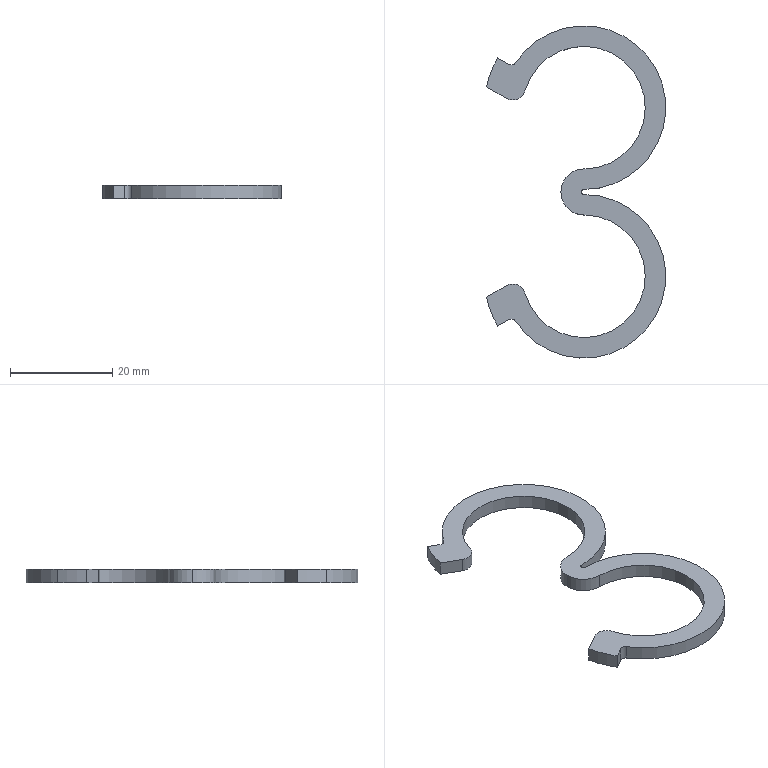Part | SolidWorks | features Extrusion 1 | 1 solid | 20 faces | box 35.068 x 65 x 2.7 mm | volume 1587 mm3 | cylinder 14 | plane 6 | commonest cylinder face diameters 1 x2 2 x2 5 x2 9 x2 24 x2 32 x2
STEP:
#1=CARTESIAN_POINT('',(-0.5,0.,2.7));
#2=VERTEX_POINT('',#1);
#3=CARTESIAN_POINT('',(0.,0.5,2.7));
#4=VERTEX_POINT('',#3);
#5=CARTESIAN_POINT('',(0.,0.,2.7));
#6=DIRECTION('',(0.,0.,-1.));
#7=DIRECTION('',(1.,0.,0.));
#8=AXIS2_PLACEMENT_3D('',#5,#6,#7);
#9=CIRCLE('',#8,0.5);
#10=EDGE_CURVE('',#2,#4,#9,.T.);
#11=ORIENTED_EDGE('',*,*,#10,.F.);
#12=CARTESIAN_POINT('',(-0.5,0.,0.));
#13=VERTEX_POINT('',#12);
#14=CARTESIAN_POINT('',(-0.5,0.,2.7));
#15=DIRECTION('',(0.,0.,-1.));
#16=VECTOR('',#15,1000.);
#17=LINE('',#14,#16);
#18=EDGE_CURVE('',#2,#13,#17,.T.);
#19=ORIENTED_EDGE('',*,*,#18,.T.);
#20=CARTESIAN_POINT('',(0.,0.5,0.));
#21=VERTEX_POINT('',#20);
#22=CARTESIAN_POINT('',(0.,0.,0.));
#23=DIRECTION('',(0.,0.,-1.));
#24=DIRECTION('',(1.,0.,0.));
#25=AXIS2_PLACEMENT_3D('',#22,#23,#24);
#26=CIRCLE('',#25,0.5);
#27=EDGE_CURVE('',#13,#21,#26,.T.);
#28=ORIENTED_EDGE('',*,*,#27,.T.);
#29=CARTESIAN_POINT('',(0.,0.5,2.7));
#30=DIRECTION('',(0.,0.,-1.));
#31=VECTOR('',#30,1000.);
#32=LINE('',#29,#31);
#33=EDGE_CURVE('',#4,#21,#32,.T.);
#34=ORIENTED_EDGE('',*,*,#33,.F.);
#35=EDGE_LOOP('',(#11,#19,#28,#34));
#36=FACE_OUTER_BOUND('',#35,.T.);
#37=CARTESIAN_POINT('',(0.,0.,2.7));
#38=DIRECTION('',(0.,0.,-1.));
#39=DIRECTION('',(-1.,0.,0.));
#40=AXIS2_PLACEMENT_3D('',#37,#38,#39);
#41=CYLINDRICAL_SURFACE('',#40,0.5);
#42=ADVANCED_FACE('',(#36),#41,.F.);
#43=CARTESIAN_POINT('',(-4.5,0.,2.7));
#44=VERTEX_POINT('',#43);
#45=CARTESIAN_POINT('',(0.,-4.5,2.7));
#46=VERTEX_POINT('',#45);
#47=CARTESIAN_POINT('',(0.,0.,2.7));
#48=DIRECTION('',(0.,0.,1.));
#49=DIRECTION('',(1.,0.,0.));
#50=AXIS2_PLACEMENT_3D('',#47,#48,#49);
#51=CIRCLE('',#50,4.5);
#52=EDGE_CURVE('',#44,#46,#51,.T.);
#53=ORIENTED_EDGE('',*,*,#52,.F.);
#54=CARTESIAN_POINT('',(-4.5,0.,0.));
#55=VERTEX_POINT('',#54);
#56=CARTESIAN_POINT('',(-4.5,0.,2.7));
#57=DIRECTION('',(0.,0.,-1.));
#58=VECTOR('',#57,1000.);
#59=LINE('',#56,#58);
#60=EDGE_CURVE('',#44,#55,#59,.T.);
#61=ORIENTED_EDGE('',*,*,#60,.T.);
#62=CARTESIAN_POINT('',(0.,-4.5,0.));
#63=VERTEX_POINT('',#62);
#64=CARTESIAN_POINT('',(0.,0.,0.));
#65=DIRECTION('',(0.,0.,1.));
#66=DIRECTION('',(1.,0.,0.));
#67=AXIS2_PLACEMENT_3D('',#64,#65,#66);
#68=CIRCLE('',#67,4.5);
#69=EDGE_CURVE('',#55,#63,#68,.T.);
#70=ORIENTED_EDGE('',*,*,#69,.T.);
#71=CARTESIAN_POINT('',(0.,-4.5,2.7));
#72=DIRECTION('',(0.,0.,-1.));
#73=VECTOR('',#72,1000.);
#74=LINE('',#71,#73);
#75=EDGE_CURVE('',#46,#63,#74,.T.);
#76=ORIENTED_EDGE('',*,*,#75,.F.);
#77=EDGE_LOOP('',(#53,#61,#70,#76));
#78=FACE_OUTER_BOUND('',#77,.T.);
#79=CARTESIAN_POINT('',(0.,0.,2.7));
#80=DIRECTION('',(0.,0.,-1.));
#81=DIRECTION('',(-1.,0.,0.));
#82=AXIS2_PLACEMENT_3D('',#79,#80,#81);
#83=CYLINDRICAL_SURFACE('',#82,4.5);
#84=ADVANCED_FACE('',(#78),#83,.T.);
#85=CARTESIAN_POINT('',(-16.887,26.25,0.));
#86=VERTEX_POINT('',#85);
#87=CARTESIAN_POINT('',(-19.068,20.581,0.));
#88=VERTEX_POINT('',#87);
#89=CARTESIAN_POINT('',(0.,16.5,0.));
#90=DIRECTION('',(0.,0.,1.));
#91=DIRECTION('',(1.,0.,0.));
#92=AXIS2_PLACEMENT_3D('',#89,#90,#91);
#93=CIRCLE('',#92,19.5);
#94=EDGE_CURVE('',#86,#88,#93,.T.);
#95=ORIENTED_EDGE('',*,*,#94,.T.);
#96=CARTESIAN_POINT('',(-19.068,20.581,2.7));
#97=VERTEX_POINT('',#96);
#98=CARTESIAN_POINT('',(-19.068,20.581,2.7));
#99=DIRECTION('',(0.,0.,-1.));
#100=VECTOR('',#99,1000.);
#101=LINE('',#98,#100);
#102=EDGE_CURVE('',#97,#88,#101,.T.);
#103=ORIENTED_EDGE('',*,*,#102,.F.);
#104=CARTESIAN_POINT('',(-16.887,26.25,2.7));
#105=VERTEX_POINT('',#104);
#106=CARTESIAN_POINT('',(0.,16.5,2.7));
#107=DIRECTION('',(0.,0.,1.));
#108=DIRECTION('',(1.,0.,0.));
#109=AXIS2_PLACEMENT_3D('',#106,#107,#108);
#110=CIRCLE('',#109,19.5);
#111=EDGE_CURVE('',#105,#97,#110,.T.);
#112=ORIENTED_EDGE('',*,*,#111,.F.);
#113=CARTESIAN_POINT('',(-16.887,26.25,2.7));
#114=DIRECTION('',(0.,0.,-1.));
#115=VECTOR('',#114,1000.);
#116=LINE('',#113,#115);
#117=EDGE_CURVE('',#105,#86,#116,.T.);
#118=ORIENTED_EDGE('',*,*,#117,.T.);
#119=EDGE_LOOP('',(#95,#103,#112,#118));
#120=FACE_OUTER_BOUND('',#119,.T.);
#121=CARTESIAN_POINT('',(0.,16.5,2.7));
#122=DIRECTION('',(0.,0.,-1.));
#123=DIRECTION('',(-1.,0.,0.));
#124=AXIS2_PLACEMENT_3D('',#121,#122,#123);
#125=CYLINDRICAL_SURFACE('',#124,19.5);
#126=ADVANCED_FACE('',(#120),#125,.T.);
#127=CARTESIAN_POINT('',(-15.186,18.339,0.));
#128=VERTEX_POINT('',#127);
#129=CARTESIAN_POINT('',(-15.186,18.339,0.));
#130=DIRECTION('',(0.866,-0.5,0.));
#131=VECTOR('',#130,1000.);
#132=LINE('',#129,#131);
#133=EDGE_CURVE('',#88,#128,#132,.T.);
#134=ORIENTED_EDGE('',*,*,#133,.T.);
#135=CARTESIAN_POINT('',(-15.186,18.339,2.7));
#136=VERTEX_POINT('',#135);
#137=CARTESIAN_POINT('',(-15.186,18.339,2.7));
#138=DIRECTION('',(0.,0.,-1.));
#139=VECTOR('',#138,1000.);
#140=LINE('',#137,#139);
#141=EDGE_CURVE('',#136,#128,#140,.T.);
#142=ORIENTED_EDGE('',*,*,#141,.F.);
#143=CARTESIAN_POINT('',(-15.186,18.339,2.7));
#144=DIRECTION('',(0.866,-0.5,0.));
#145=VECTOR('',#144,1000.);
#146=LINE('',#143,#145);
#147=EDGE_CURVE('',#97,#136,#146,.T.);
#148=ORIENTED_EDGE('',*,*,#147,.F.);
#149=ORIENTED_EDGE('',*,*,#102,.T.);
#150=EDGE_LOOP('',(#134,#142,#148,#149));
#151=FACE_OUTER_BOUND('',#150,.T.);
#152=CARTESIAN_POINT('',(-15.186,18.339,2.7));
#153=DIRECTION('',(0.5,0.866,0.));
#154=DIRECTION('',(-0.866,0.5,0.));
#155=AXIS2_PLACEMENT_3D('',#152,#153,#154);
#156=PLANE('',#155);
#157=ADVANCED_FACE('',(#151),#156,.F.);
#158=CARTESIAN_POINT('',(-11.533,19.814,0.));
#159=VERTEX_POINT('',#158);
#160=CARTESIAN_POINT('',(-13.936,20.505,0.));
#161=DIRECTION('',(0.,0.,1.));
#162=DIRECTION('',(-1.,0.,0.));
#163=AXIS2_PLACEMENT_3D('',#160,#161,#162);
#164=CIRCLE('',#163,2.5);
#165=EDGE_CURVE('',#128,#159,#164,.T.);
#166=ORIENTED_EDGE('',*,*,#165,.T.);
#167=CARTESIAN_POINT('',(-11.533,19.814,2.7));
#168=VERTEX_POINT('',#167);
#169=CARTESIAN_POINT('',(-11.533,19.814,2.7));
#170=DIRECTION('',(0.,0.,-1.));
#171=VECTOR('',#170,1000.);
#172=LINE('',#169,#171);
#173=EDGE_CURVE('',#168,#159,#172,.T.);
#174=ORIENTED_EDGE('',*,*,#173,.F.);
#175=CARTESIAN_POINT('',(-13.936,20.505,2.7));
#176=DIRECTION('',(0.,0.,1.));
#177=DIRECTION('',(-1.,0.,0.));
#178=AXIS2_PLACEMENT_3D('',#175,#176,#177);
#179=CIRCLE('',#178,2.5);
#180=EDGE_CURVE('',#136,#168,#179,.T.);
#181=ORIENTED_EDGE('',*,*,#180,.F.);
#182=ORIENTED_EDGE('',*,*,#141,.T.);
#183=EDGE_LOOP('',(#166,#174,#181,#182));
#184=FACE_OUTER_BOUND('',#183,.T.);
#185=CARTESIAN_POINT('',(-13.936,20.505,2.7));
#186=DIRECTION('',(0.,0.,-1.));
#187=DIRECTION('',(-1.,0.,0.));
#188=AXIS2_PLACEMENT_3D('',#185,#186,#187);
#189=CYLINDRICAL_SURFACE('',#188,2.5);
#190=ADVANCED_FACE('',(#184),#189,.T.);
#191=CARTESIAN_POINT('',(0.,4.5,0.));
#192=VERTEX_POINT('',#191);
#193=CARTESIAN_POINT('',(0.,16.5,0.));
#194=DIRECTION('',(0.,0.,-1.));
#195=DIRECTION('',(1.,0.,0.));
#196=AXIS2_PLACEMENT_3D('',#193,#194,#195);
#197=CIRCLE('',#196,12.);
#198=EDGE_CURVE('',#159,#192,#197,.T.);
#199=ORIENTED_EDGE('',*,*,#198,.T.);
#200=CARTESIAN_POINT('',(0.,4.5,2.7));
#201=VERTEX_POINT('',#200);
#202=CARTESIAN_POINT('',(0.,4.5,2.7));
#203=DIRECTION('',(0.,0.,-1.));
#204=VECTOR('',#203,1000.);
#205=LINE('',#202,#204);
#206=EDGE_CURVE('',#201,#192,#205,.T.);
#207=ORIENTED_EDGE('',*,*,#206,.F.);
#208=CARTESIAN_POINT('',(0.,16.5,2.7));
#209=DIRECTION('',(0.,0.,-1.));
#210=DIRECTION('',(1.,0.,0.));
#211=AXIS2_PLACEMENT_3D('',#208,#209,#210);
#212=CIRCLE('',#211,12.);
#213=EDGE_CURVE('',#168,#201,#212,.T.);
#214=ORIENTED_EDGE('',*,*,#213,.F.);
#215=ORIENTED_EDGE('',*,*,#173,.T.);
#216=EDGE_LOOP('',(#199,#207,#214,#215));
#217=FACE_OUTER_BOUND('',#216,.T.);
#218=CARTESIAN_POINT('',(0.,16.5,2.7));
#219=DIRECTION('',(0.,0.,-1.));
#220=DIRECTION('',(-1.,0.,0.));
#221=AXIS2_PLACEMENT_3D('',#218,#219,#220);
#222=CYLINDRICAL_SURFACE('',#221,12.);
#223=ADVANCED_FACE('',(#217),#222,.F.);
#224=ORIENTED_EDGE('',*,*,#60,.F.);
#225=CARTESIAN_POINT('',(0.,0.,2.7));
#226=DIRECTION('',(0.,0.,1.));
#227=DIRECTION('',(1.,0.,0.));
#228=AXIS2_PLACEMENT_3D('',#225,#226,#227);
#229=CIRCLE('',#228,4.5);
#230=EDGE_CURVE('',#201,#44,#229,.T.);
#231=ORIENTED_EDGE('',*,*,#230,.F.);
#232=ORIENTED_EDGE('',*,*,#206,.T.);
#233=CARTESIAN_POINT('',(0.,0.,0.));
#234=DIRECTION('',(0.,0.,1.));
#235=DIRECTION('',(1.,0.,0.));
#236=AXIS2_PLACEMENT_3D('',#233,#234,#235);
#237=CIRCLE('',#236,4.5);
#238=EDGE_CURVE('',#192,#55,#237,.T.);
#239=ORIENTED_EDGE('',*,*,#238,.T.);
#240=EDGE_LOOP('',(#224,#231,#232,#239));
#241=FACE_OUTER_BOUND('',#240,.T.);
#242=CARTESIAN_POINT('',(0.,0.,2.7));
#243=DIRECTION('',(0.,0.,-1.));
#244=DIRECTION('',(-1.,0.,0.));
#245=AXIS2_PLACEMENT_3D('',#242,#243,#244);
#246=CYLINDRICAL_SURFACE('',#245,4.5);
#247=ADVANCED_FACE('',(#241),#246,.T.);
#248=CARTESIAN_POINT('',(-11.533,-19.814,0.));
#249=VERTEX_POINT('',#248);
#250=CARTESIAN_POINT('',(0.,-16.5,0.));
#251=DIRECTION('',(0.,0.,-1.));
#252=DIRECTION('',(-1.,0.,0.));
#253=AXIS2_PLACEMENT_3D('',#250,#251,#252);
#254=CIRCLE('',#253,12.);
#255=EDGE_CURVE('',#63,#249,#254,.T.);
#256=ORIENTED_EDGE('',*,*,#255,.T.);
#257=CARTESIAN_POINT('',(-11.533,-19.814,2.7));
#258=VERTEX_POINT('',#257);
#259=CARTESIAN_POINT('',(-11.533,-19.814,2.7));
#260=DIRECTION('',(0.,0.,-1.));
#261=VECTOR('',#260,1000.);
#262=LINE('',#259,#261);
#263=EDGE_CURVE('',#258,#249,#262,.T.);
#264=ORIENTED_EDGE('',*,*,#263,.F.);
#265=CARTESIAN_POINT('',(0.,-16.5,2.7));
#266=DIRECTION('',(0.,0.,-1.));
#267=DIRECTION('',(-1.,0.,0.));
#268=AXIS2_PLACEMENT_3D('',#265,#266,#267);
#269=CIRCLE('',#268,12.);
#270=EDGE_CURVE('',#46,#258,#269,.T.);
#271=ORIENTED_EDGE('',*,*,#270,.F.);
#272=ORIENTED_EDGE('',*,*,#75,.T.);
#273=EDGE_LOOP('',(#256,#264,#271,#272));
#274=FACE_OUTER_BOUND('',#273,.T.);
#275=CARTESIAN_POINT('',(0.,-16.5,2.7));
#276=DIRECTION('',(0.,0.,-1.));
#277=DIRECTION('',(-1.,0.,0.));
#278=AXIS2_PLACEMENT_3D('',#275,#276,#277);
#279=CYLINDRICAL_SURFACE('',#278,12.);
#280=ADVANCED_FACE('',(#274),#279,.F.);
#281=CARTESIAN_POINT('',(-15.186,-18.339,0.));
#282=VERTEX_POINT('',#281);
#283=CARTESIAN_POINT('',(-13.936,-20.505,0.));
#284=DIRECTION('',(0.,0.,1.));
#285=DIRECTION('',(1.,0.,0.));
#286=AXIS2_PLACEMENT_3D('',#283,#284,#285);
#287=CIRCLE('',#286,2.5);
#288=EDGE_CURVE('',#249,#282,#287,.T.);
#289=ORIENTED_EDGE('',*,*,#288,.T.);
#290=CARTESIAN_POINT('',(-15.186,-18.339,2.7));
#291=VERTEX_POINT('',#290);
#292=CARTESIAN_POINT('',(-15.186,-18.339,2.7));
#293=DIRECTION('',(0.,0.,-1.));
#294=VECTOR('',#293,1000.);
#295=LINE('',#292,#294);
#296=EDGE_CURVE('',#291,#282,#295,.T.);
#297=ORIENTED_EDGE('',*,*,#296,.F.);
#298=CARTESIAN_POINT('',(-13.936,-20.505,2.7));
#299=DIRECTION('',(0.,0.,1.));
#300=DIRECTION('',(1.,0.,0.));
#301=AXIS2_PLACEMENT_3D('',#298,#299,#300);
#302=CIRCLE('',#301,2.5);
#303=EDGE_CURVE('',#258,#291,#302,.T.);
#304=ORIENTED_EDGE('',*,*,#303,.F.);
#305=ORIENTED_EDGE('',*,*,#263,.T.);
#306=EDGE_LOOP('',(#289,#297,#304,#305));
#307=FACE_OUTER_BOUND('',#306,.T.);
#308=CARTESIAN_POINT('',(-13.936,-20.505,2.7));
#309=DIRECTION('',(0.,0.,-1.));
#310=DIRECTION('',(-1.,0.,0.));
#311=AXIS2_PLACEMENT_3D('',#308,#309,#310);
#312=CYLINDRICAL_SURFACE('',#311,2.5);
#313=ADVANCED_FACE('',(#307),#312,.T.);
#314=CARTESIAN_POINT('',(-19.068,-20.581,0.));
#315=VERTEX_POINT('',#314);
#316=CARTESIAN_POINT('',(-15.186,-18.339,0.));
#317=DIRECTION('',(-0.866,-0.5,0.));
#318=VECTOR('',#317,1000.);
#319=LINE('',#316,#318);
#320=EDGE_CURVE('',#282,#315,#319,.T.);
#321=ORIENTED_EDGE('',*,*,#320,.T.);
#322=CARTESIAN_POINT('',(-19.068,-20.581,2.7));
#323=VERTEX_POINT('',#322);
#324=CARTESIAN_POINT('',(-19.068,-20.581,2.7));
#325=DIRECTION('',(0.,0.,-1.));
#326=VECTOR('',#325,1000.);
#327=LINE('',#324,#326);
#328=EDGE_CURVE('',#323,#315,#327,.T.);
#329=ORIENTED_EDGE('',*,*,#328,.F.);
#330=CARTESIAN_POINT('',(-15.186,-18.339,2.7));
#331=DIRECTION('',(-0.866,-0.5,0.));
#332=VECTOR('',#331,1000.);
#333=LINE('',#330,#332);
#334=EDGE_CURVE('',#291,#323,#333,.T.);
#335=ORIENTED_EDGE('',*,*,#334,.F.);
#336=ORIENTED_EDGE('',*,*,#296,.T.);
#337=EDGE_LOOP('',(#321,#329,#335,#336));
#338=FACE_OUTER_BOUND('',#337,.T.);
#339=CARTESIAN_POINT('',(-15.186,-18.339,2.7));
#340=DIRECTION('',(0.5,-0.866,0.));
#341=DIRECTION('',(0.866,0.5,0.));
#342=AXIS2_PLACEMENT_3D('',#339,#340,#341);
#343=PLANE('',#342);
#344=ADVANCED_FACE('',(#338),#343,.F.);
#345=CARTESIAN_POINT('',(-16.887,-26.25,0.));
#346=VERTEX_POINT('',#345);
#347=CARTESIAN_POINT('',(0.,-16.5,0.));
#348=DIRECTION('',(0.,0.,1.));
#349=DIRECTION('',(-1.,0.,0.));
#350=AXIS2_PLACEMENT_3D('',#347,#348,#349);
#351=CIRCLE('',#350,19.5);
#352=EDGE_CURVE('',#315,#346,#351,.T.);
#353=ORIENTED_EDGE('',*,*,#352,.T.);
#354=CARTESIAN_POINT('',(-16.887,-26.25,2.7));
#355=VERTEX_POINT('',#354);
#356=CARTESIAN_POINT('',(-16.887,-26.25,2.7));
#357=DIRECTION('',(0.,0.,-1.));
#358=VECTOR('',#357,1000.);
#359=LINE('',#356,#358);
#360=EDGE_CURVE('',#355,#346,#359,.T.);
#361=ORIENTED_EDGE('',*,*,#360,.F.);
#362=CARTESIAN_POINT('',(0.,-16.5,2.7));
#363=DIRECTION('',(0.,0.,1.));
#364=DIRECTION('',(-1.,0.,0.));
#365=AXIS2_PLACEMENT_3D('',#362,#363,#364);
#366=CIRCLE('',#365,19.5);
#367=EDGE_CURVE('',#323,#355,#366,.T.);
#368=ORIENTED_EDGE('',*,*,#367,.F.);
#369=ORIENTED_EDGE('',*,*,#328,.T.);
#370=EDGE_LOOP('',(#353,#361,#368,#369));
#371=FACE_OUTER_BOUND('',#370,.T.);
#372=CARTESIAN_POINT('',(0.,-16.5,2.7));
#373=DIRECTION('',(0.,0.,-1.));
#374=DIRECTION('',(-1.,0.,0.));
#375=AXIS2_PLACEMENT_3D('',#372,#373,#374);
#376=CYLINDRICAL_SURFACE('',#375,19.5);
#377=ADVANCED_FACE('',(#371),#376,.T.);
#378=CARTESIAN_POINT('',(-14.697,-24.985,0.));
#379=VERTEX_POINT('',#378);
#380=CARTESIAN_POINT('',(-14.697,-24.985,0.));
#381=DIRECTION('',(0.866,0.5,0.));
#382=VECTOR('',#381,1000.);
#383=LINE('',#380,#382);
#384=EDGE_CURVE('',#346,#379,#383,.T.);
#385=ORIENTED_EDGE('',*,*,#384,.T.);
#386=CARTESIAN_POINT('',(-14.697,-24.985,2.7));
#387=VERTEX_POINT('',#386);
#388=CARTESIAN_POINT('',(-14.697,-24.985,2.7));
#389=DIRECTION('',(0.,0.,-1.));
#390=VECTOR('',#389,1000.);
#391=LINE('',#388,#390);
#392=EDGE_CURVE('',#387,#379,#391,.T.);
#393=ORIENTED_EDGE('',*,*,#392,.F.);
#394=CARTESIAN_POINT('',(-14.697,-24.985,2.7));
#395=DIRECTION('',(0.866,0.5,0.));
#396=VECTOR('',#395,1000.);
#397=LINE('',#394,#396);
#398=EDGE_CURVE('',#355,#387,#397,.T.);
#399=ORIENTED_EDGE('',*,*,#398,.F.);
#400=ORIENTED_EDGE('',*,*,#360,.T.);
#401=EDGE_LOOP('',(#385,#393,#399,#400));
#402=FACE_OUTER_BOUND('',#401,.T.);
#403=CARTESIAN_POINT('',(-14.697,-24.985,2.7));
#404=DIRECTION('',(-0.5,0.866,0.));
#405=DIRECTION('',(-0.866,-0.5,0.));
#406=AXIS2_PLACEMENT_3D('',#403,#404,#405);
#407=PLANE('',#406);
#408=ADVANCED_FACE('',(#402),#407,.F.);
#409=CARTESIAN_POINT('',(-13.362,-25.301,0.));
#410=VERTEX_POINT('',#409);
#411=CARTESIAN_POINT('',(-14.197,-25.851,0.));
#412=DIRECTION('',(0.,0.,-1.));
#413=DIRECTION('',(1.,0.,0.));
#414=AXIS2_PLACEMENT_3D('',#411,#412,#413);
#415=CIRCLE('',#414,1.);
#416=EDGE_CURVE('',#379,#410,#415,.T.);
#417=ORIENTED_EDGE('',*,*,#416,.T.);
#418=CARTESIAN_POINT('',(-13.362,-25.301,2.7));
#419=VERTEX_POINT('',#418);
#420=CARTESIAN_POINT('',(-13.362,-25.301,2.7));
#421=DIRECTION('',(0.,0.,-1.));
#422=VECTOR('',#421,1000.);
#423=LINE('',#420,#422);
#424=EDGE_CURVE('',#419,#410,#423,.T.);
#425=ORIENTED_EDGE('',*,*,#424,.F.);
#426=CARTESIAN_POINT('',(-14.197,-25.851,2.7));
#427=DIRECTION('',(0.,0.,-1.));
#428=DIRECTION('',(1.,0.,0.));
#429=AXIS2_PLACEMENT_3D('',#426,#427,#428);
#430=CIRCLE('',#429,1.);
#431=EDGE_CURVE('',#387,#419,#430,.T.);
#432=ORIENTED_EDGE('',*,*,#431,.F.);
#433=ORIENTED_EDGE('',*,*,#392,.T.);
#434=EDGE_LOOP('',(#417,#425,#432,#433));
#435=FACE_OUTER_BOUND('',#434,.T.);
#436=CARTESIAN_POINT('',(-14.197,-25.851,2.7));
#437=DIRECTION('',(0.,0.,-1.));
#438=DIRECTION('',(-1.,0.,0.));
#439=AXIS2_PLACEMENT_3D('',#436,#437,#438);
#440=CYLINDRICAL_SURFACE('',#439,1.);
#441=ADVANCED_FACE('',(#435),#440,.F.);
#442=CARTESIAN_POINT('',(0.,-0.5,0.));
#443=VERTEX_POINT('',#442);
#444=CARTESIAN_POINT('',(0.,-16.5,0.));
#445=DIRECTION('',(0.,0.,1.));
#446=DIRECTION('',(-1.,0.,0.));
#447=AXIS2_PLACEMENT_3D('',#444,#445,#446);
#448=CIRCLE('',#447,16.);
#449=EDGE_CURVE('',#410,#443,#448,.T.);
#450=ORIENTED_EDGE('',*,*,#449,.T.);
#451=CARTESIAN_POINT('',(0.,-0.5,2.7));
#452=VERTEX_POINT('',#451);
#453=CARTESIAN_POINT('',(0.,-0.5,2.7));
#454=DIRECTION('',(0.,0.,-1.));
#455=VECTOR('',#454,1000.);
#456=LINE('',#453,#455);
#457=EDGE_CURVE('',#452,#443,#456,.T.);
#458=ORIENTED_EDGE('',*,*,#457,.F.);
#459=CARTESIAN_POINT('',(0.,-16.5,2.7));
#460=DIRECTION('',(0.,0.,1.));
#461=DIRECTION('',(-1.,0.,0.));
#462=AXIS2_PLACEMENT_3D('',#459,#460,#461);
#463=CIRCLE('',#462,16.);
#464=EDGE_CURVE('',#419,#452,#463,.T.);
#465=ORIENTED_EDGE('',*,*,#464,.F.);
#466=ORIENTED_EDGE('',*,*,#424,.T.);
#467=EDGE_LOOP('',(#450,#458,#465,#466));
#468=FACE_OUTER_BOUND('',#467,.T.);
#469=CARTESIAN_POINT('',(0.,-16.5,2.7));
#470=DIRECTION('',(0.,0.,-1.));
#471=DIRECTION('',(-1.,0.,0.));
#472=AXIS2_PLACEMENT_3D('',#469,#470,#471);
#473=CYLINDRICAL_SURFACE('',#472,16.);
#474=ADVANCED_FACE('',(#468),#473,.T.);
#475=ORIENTED_EDGE('',*,*,#18,.F.);
#476=CARTESIAN_POINT('',(0.,0.,2.7));
#477=DIRECTION('',(0.,0.,-1.));
#478=DIRECTION('',(1.,0.,0.));
#479=AXIS2_PLACEMENT_3D('',#476,#477,#478);
#480=CIRCLE('',#479,0.5);
#481=EDGE_CURVE('',#452,#2,#480,.T.);
#482=ORIENTED_EDGE('',*,*,#481,.F.);
#483=ORIENTED_EDGE('',*,*,#457,.T.);
#484=CARTESIAN_POINT('',(0.,0.,0.));
#485=DIRECTION('',(0.,0.,-1.));
#486=DIRECTION('',(1.,0.,0.));
#487=AXIS2_PLACEMENT_3D('',#484,#485,#486);
#488=CIRCLE('',#487,0.5);
#489=EDGE_CURVE('',#443,#13,#488,.T.);
#490=ORIENTED_EDGE('',*,*,#489,.T.);
#491=EDGE_LOOP('',(#475,#482,#483,#490));
#492=FACE_OUTER_BOUND('',#491,.T.);
#493=CARTESIAN_POINT('',(0.,0.,2.7));
#494=DIRECTION('',(0.,0.,-1.));
#495=DIRECTION('',(-1.,0.,0.));
#496=AXIS2_PLACEMENT_3D('',#493,#494,#495);
#497=CYLINDRICAL_SURFACE('',#496,0.5);
#498=ADVANCED_FACE('',(#492),#497,.F.);
#499=CARTESIAN_POINT('',(-13.362,25.301,0.));
#500=VERTEX_POINT('',#499);
#501=CARTESIAN_POINT('',(0.,16.5,0.));
#502=DIRECTION('',(0.,0.,1.));
#503=DIRECTION('',(1.,0.,0.));
#504=AXIS2_PLACEMENT_3D('',#501,#502,#503);
#505=CIRCLE('',#504,16.);
#506=EDGE_CURVE('',#21,#500,#505,.T.);
#507=ORIENTED_EDGE('',*,*,#506,.T.);
#508=CARTESIAN_POINT('',(-13.362,25.301,2.7));
#509=VERTEX_POINT('',#508);
#510=CARTESIAN_POINT('',(-13.362,25.301,2.7));
#511=DIRECTION('',(0.,0.,-1.));
#512=VECTOR('',#511,1000.);
#513=LINE('',#510,#512);
#514=EDGE_CURVE('',#509,#500,#513,.T.);
#515=ORIENTED_EDGE('',*,*,#514,.F.);
#516=CARTESIAN_POINT('',(0.,16.5,2.7));
#517=DIRECTION('',(0.,0.,1.));
#518=DIRECTION('',(1.,0.,0.));
#519=AXIS2_PLACEMENT_3D('',#516,#517,#518);
#520=CIRCLE('',#519,16.);
#521=EDGE_CURVE('',#4,#509,#520,.T.);
#522=ORIENTED_EDGE('',*,*,#521,.F.);
#523=ORIENTED_EDGE('',*,*,#33,.T.);
#524=EDGE_LOOP('',(#507,#515,#522,#523));
#525=FACE_OUTER_BOUND('',#524,.T.);
#526=CARTESIAN_POINT('',(0.,16.5,2.7));
#527=DIRECTION('',(0.,0.,-1.));
#528=DIRECTION('',(-1.,0.,0.));
#529=AXIS2_PLACEMENT_3D('',#526,#527,#528);
#530=CYLINDRICAL_SURFACE('',#529,16.);
#531=ADVANCED_FACE('',(#525),#530,.T.);
#532=CARTESIAN_POINT('',(-14.697,24.985,0.));
#533=VERTEX_POINT('',#532);
#534=CARTESIAN_POINT('',(-14.197,25.851,0.));
#535=DIRECTION('',(0.,0.,-1.));
#536=DIRECTION('',(-1.,0.,0.));
#537=AXIS2_PLACEMENT_3D('',#534,#535,#536);
#538=CIRCLE('',#537,1.);
#539=EDGE_CURVE('',#500,#533,#538,.T.);
#540=ORIENTED_EDGE('',*,*,#539,.T.);
#541=CARTESIAN_POINT('',(-14.697,24.985,2.7));
#542=VERTEX_POINT('',#541);
#543=CARTESIAN_POINT('',(-14.697,24.985,2.7));
#544=DIRECTION('',(0.,0.,-1.));
#545=VECTOR('',#544,1000.);
#546=LINE('',#543,#545);
#547=EDGE_CURVE('',#542,#533,#546,.T.);
#548=ORIENTED_EDGE('',*,*,#547,.F.);
#549=CARTESIAN_POINT('',(-14.197,25.851,2.7));
#550=DIRECTION('',(0.,0.,-1.));
#551=DIRECTION('',(-1.,0.,0.));
#552=AXIS2_PLACEMENT_3D('',#549,#550,#551);
#553=CIRCLE('',#552,1.);
#554=EDGE_CURVE('',#509,#542,#553,.T.);
#555=ORIENTED_EDGE('',*,*,#554,.F.);
#556=ORIENTED_EDGE('',*,*,#514,.T.);
#557=EDGE_LOOP('',(#540,#548,#555,#556));
#558=FACE_OUTER_BOUND('',#557,.T.);
#559=CARTESIAN_POINT('',(-14.197,25.851,2.7));
#560=DIRECTION('',(0.,0.,-1.));
#561=DIRECTION('',(-1.,0.,0.));
#562=AXIS2_PLACEMENT_3D('',#559,#560,#561);
#563=CYLINDRICAL_SURFACE('',#562,1.);
#564=ADVANCED_FACE('',(#558),#563,.F.);
#565=CARTESIAN_POINT('',(-14.697,24.985,0.));
#566=DIRECTION('',(-0.866,0.5,0.));
#567=VECTOR('',#566,1000.);
#568=LINE('',#565,#567);
#569=EDGE_CURVE('',#533,#86,#568,.T.);
#570=ORIENTED_EDGE('',*,*,#569,.T.);
#571=ORIENTED_EDGE('',*,*,#117,.F.);
#572=CARTESIAN_POINT('',(-14.697,24.985,2.7));
#573=DIRECTION('',(-0.866,0.5,0.));
#574=VECTOR('',#573,1000.);
#575=LINE('',#572,#574);
#576=EDGE_CURVE('',#542,#105,#575,.T.);
#577=ORIENTED_EDGE('',*,*,#576,.F.);
#578=ORIENTED_EDGE('',*,*,#547,.T.);
#579=EDGE_LOOP('',(#570,#571,#577,#578));
#580=FACE_OUTER_BOUND('',#579,.T.);
#581=CARTESIAN_POINT('',(-14.697,24.985,2.7));
#582=DIRECTION('',(-0.5,-0.866,0.));
#583=DIRECTION('',(0.866,-0.5,0.));
#584=AXIS2_PLACEMENT_3D('',#581,#582,#583);
#585=PLANE('',#584);
#586=ADVANCED_FACE('',(#580),#585,.F.);
#587=ORIENTED_EDGE('',*,*,#111,.T.);
#588=ORIENTED_EDGE('',*,*,#147,.T.);
#589=ORIENTED_EDGE('',*,*,#180,.T.);
#590=ORIENTED_EDGE('',*,*,#213,.T.);
#591=ORIENTED_EDGE('',*,*,#230,.T.);
#592=ORIENTED_EDGE('',*,*,#52,.T.);
#593=ORIENTED_EDGE('',*,*,#270,.T.);
#594=ORIENTED_EDGE('',*,*,#303,.T.);
#595=ORIENTED_EDGE('',*,*,#334,.T.);
#596=ORIENTED_EDGE('',*,*,#367,.T.);
#597=ORIENTED_EDGE('',*,*,#398,.T.);
#598=ORIENTED_EDGE('',*,*,#431,.T.);
#599=ORIENTED_EDGE('',*,*,#464,.T.);
#600=ORIENTED_EDGE('',*,*,#481,.T.);
#601=ORIENTED_EDGE('',*,*,#10,.T.);
#602=ORIENTED_EDGE('',*,*,#521,.T.);
#603=ORIENTED_EDGE('',*,*,#554,.T.);
#604=ORIENTED_EDGE('',*,*,#576,.T.);
#605=EDGE_LOOP('',(#587,#588,#589,#590,#591,#592,#593,#594,#595,#596,#597,#598,#599,#600,#601,#602,#603,#604));
#606=FACE_OUTER_BOUND('',#605,.T.);
#607=CARTESIAN_POINT('',(0.,16.5,2.7));
#608=DIRECTION('',(0.,0.,1.));
#609=DIRECTION('',(1.,0.,0.));
#610=AXIS2_PLACEMENT_3D('',#607,#608,#609);
#611=PLANE('',#610);
#612=ADVANCED_FACE('',(#606),#611,.T.);
#613=ORIENTED_EDGE('',*,*,#94,.F.);
#614=ORIENTED_EDGE('',*,*,#569,.F.);
#615=ORIENTED_EDGE('',*,*,#539,.F.);
#616=ORIENTED_EDGE('',*,*,#506,.F.);
#617=ORIENTED_EDGE('',*,*,#27,.F.);
#618=ORIENTED_EDGE('',*,*,#489,.F.);
#619=ORIENTED_EDGE('',*,*,#449,.F.);
#620=ORIENTED_EDGE('',*,*,#416,.F.);
#621=ORIENTED_EDGE('',*,*,#384,.F.);
#622=ORIENTED_EDGE('',*,*,#352,.F.);
#623=ORIENTED_EDGE('',*,*,#320,.F.);
#624=ORIENTED_EDGE('',*,*,#288,.F.);
#625=ORIENTED_EDGE('',*,*,#255,.F.);
#626=ORIENTED_EDGE('',*,*,#69,.F.);
#627=ORIENTED_EDGE('',*,*,#238,.F.);
#628=ORIENTED_EDGE('',*,*,#198,.F.);
#629=ORIENTED_EDGE('',*,*,#165,.F.);
#630=ORIENTED_EDGE('',*,*,#133,.F.);
#631=EDGE_LOOP('',(#613,#614,#615,#616,#617,#618,#619,#620,#621,#622,#623,#624,#625,#626,#627,#628,#629,#630));
#632=FACE_OUTER_BOUND('',#631,.T.);
#633=CARTESIAN_POINT('',(0.,16.5,0.));
#634=DIRECTION('',(0.,0.,1.));
#635=DIRECTION('',(1.,0.,0.));
#636=AXIS2_PLACEMENT_3D('',#633,#634,#635);
#637=PLANE('',#636);
#638=ADVANCED_FACE('',(#632),#637,.F.);
#639=CLOSED_SHELL('',(#42,#84,#126,#157,#190,#223,#247,#280,#313,#344,#377,#408,#441,#474,#498,#531,#564,#586,#612,#638));
#640=MANIFOLD_SOLID_BREP('',#639);
#641=CARTESIAN_POINT('',(0.,0.,0.));
#642=DIRECTION('',(0.,0.,1.));
#643=DIRECTION('',(1.,0.,0.));
#644=AXIS2_PLACEMENT_3D('',#641,#642,#643);
#645=(LENGTH_UNIT()NAMED_UNIT(*)SI_UNIT(.MILLI.,.METRE.));
#646=UNCERTAINTY_MEASURE_WITH_UNIT(LENGTH_MEASURE(0.00001),#645,'','');
#647=(NAMED_UNIT(*)PLANE_ANGLE_UNIT()SI_UNIT($,.RADIAN.));
#648=(NAMED_UNIT(*)SI_UNIT($,.STERADIAN.)SOLID_ANGLE_UNIT());
#649=(GEOMETRIC_REPRESENTATION_CONTEXT(3)GLOBAL_UNCERTAINTY_ASSIGNED_CONTEXT((#646))GLOBAL_UNIT_ASSIGNED_CONTEXT((#645,#647,#648))REPRESENTATION_CONTEXT('',''));
#650=ADVANCED_BREP_SHAPE_REPRESENTATION('',(#640,#644),#649);